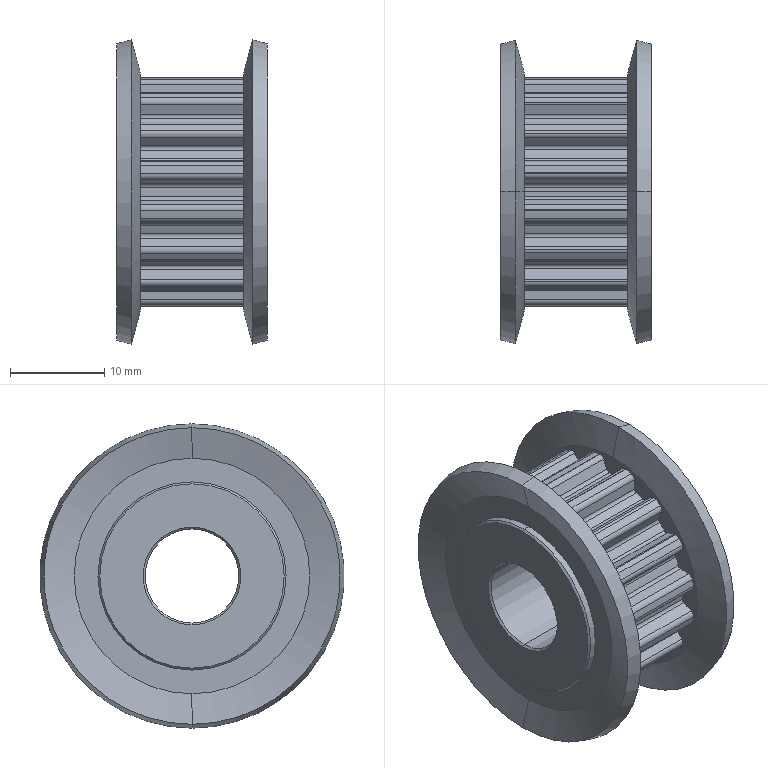Part | SolidWorks | features ICE 1, Revolution 1 | 1 solid | 169 faces | box 16 x 32.358 x 32.358 mm | volume 6392 mm3 | cylinder 115 | plane 38 | cone 16 | commonest cylinder face diameters 0.8 x38 1.2 x38 21 x17 24.6 x16 20 x4 10 x2